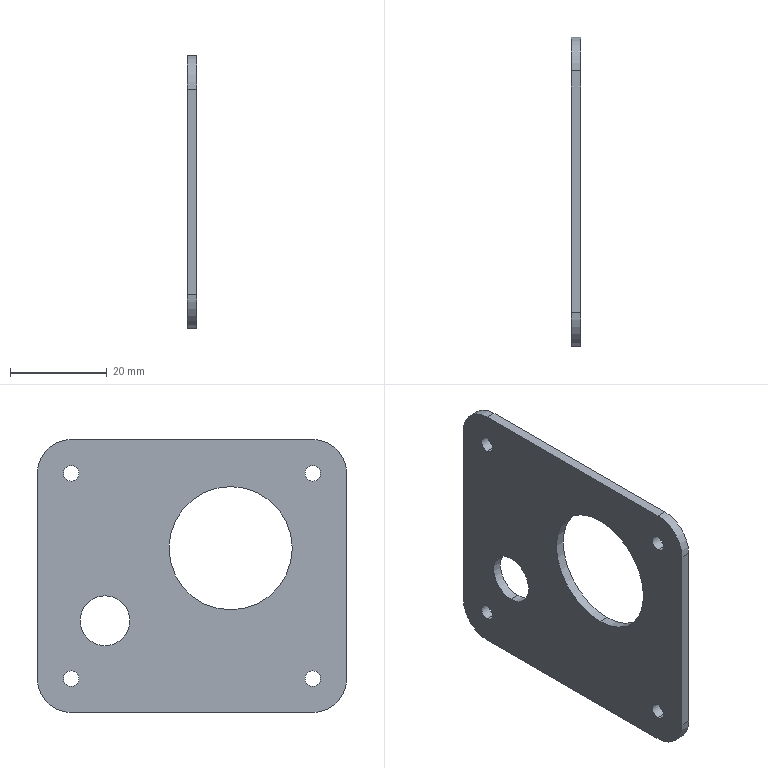Part | SolidWorks | features BaseBody 1 | 1 solid | 22 faces | box 2 x 64 x 56.5 mm | volume 5895 mm3 | cylinder 16 | plane 6 | commonest cylinder face diameters 3.2 x8 14 x4 10.3 x2 25.5 x2
STEP:
#1=CARTESIAN_POINT('',(-238.,130.5,52.4));
#2=VERTEX_POINT('',#1);
#3=CARTESIAN_POINT('',(-238.,130.5,55.6));
#4=VERTEX_POINT('',#3);
#5=CARTESIAN_POINT('',(-238.,130.5,54.));
#6=DIRECTION('',(-1.,0.,0.));
#7=DIRECTION('',(0.,0.,1.));
#8=AXIS2_PLACEMENT_3D('',#5,#6,#7);
#9=CIRCLE('',#8,1.6);
#10=EDGE_CURVE('',#2,#4,#9,.T.);
#11=ORIENTED_EDGE('',*,*,#10,.F.);
#12=CARTESIAN_POINT('',(-240.,130.5,52.4));
#13=VERTEX_POINT('',#12);
#14=CARTESIAN_POINT('',(-228.95,130.5,52.4));
#15=DIRECTION('',(-1.,0.,0.));
#16=VECTOR('',#15,1000.);
#17=LINE('',#14,#16);
#18=EDGE_CURVE('',#2,#13,#17,.T.);
#19=ORIENTED_EDGE('',*,*,#18,.T.);
#20=CARTESIAN_POINT('',(-240.,130.5,55.6));
#21=VERTEX_POINT('',#20);
#22=CARTESIAN_POINT('',(-240.,130.5,54.));
#23=DIRECTION('',(1.,0.,0.));
#24=DIRECTION('',(0.,0.,1.));
#25=AXIS2_PLACEMENT_3D('',#22,#23,#24);
#26=CIRCLE('',#25,1.6);
#27=EDGE_CURVE('',#21,#13,#26,.T.);
#28=ORIENTED_EDGE('',*,*,#27,.F.);
#29=CARTESIAN_POINT('',(-228.95,130.5,55.6));
#30=DIRECTION('',(-1.,0.,0.));
#31=VECTOR('',#30,1000.);
#32=LINE('',#29,#31);
#33=EDGE_CURVE('',#4,#21,#32,.T.);
#34=ORIENTED_EDGE('',*,*,#33,.F.);
#35=EDGE_LOOP('',(#11,#19,#28,#34));
#36=FACE_OUTER_BOUND('',#35,.T.);
#37=CARTESIAN_POINT('',(-228.95,130.5,54.));
#38=DIRECTION('',(-1.,0.,0.));
#39=DIRECTION('',(0.,0.,1.));
#40=AXIS2_PLACEMENT_3D('',#37,#38,#39);
#41=CYLINDRICAL_SURFACE('',#40,1.6);
#42=ADVANCED_FACE('',(#36),#41,.F.);
#43=CARTESIAN_POINT('',(-238.,80.5,9.9));
#44=VERTEX_POINT('',#43);
#45=CARTESIAN_POINT('',(-238.,80.5,13.1));
#46=VERTEX_POINT('',#45);
#47=CARTESIAN_POINT('',(-238.,80.5,11.5));
#48=DIRECTION('',(-1.,0.,0.));
#49=DIRECTION('',(0.,0.,1.));
#50=AXIS2_PLACEMENT_3D('',#47,#48,#49);
#51=CIRCLE('',#50,1.6);
#52=EDGE_CURVE('',#44,#46,#51,.T.);
#53=ORIENTED_EDGE('',*,*,#52,.F.);
#54=CARTESIAN_POINT('',(-240.,80.5,9.9));
#55=VERTEX_POINT('',#54);
#56=CARTESIAN_POINT('',(-228.95,80.5,9.9));
#57=DIRECTION('',(-1.,0.,0.));
#58=VECTOR('',#57,1000.);
#59=LINE('',#56,#58);
#60=EDGE_CURVE('',#44,#55,#59,.T.);
#61=ORIENTED_EDGE('',*,*,#60,.T.);
#62=CARTESIAN_POINT('',(-240.,80.5,13.1));
#63=VERTEX_POINT('',#62);
#64=CARTESIAN_POINT('',(-240.,80.5,11.5));
#65=DIRECTION('',(1.,0.,0.));
#66=DIRECTION('',(0.,0.,1.));
#67=AXIS2_PLACEMENT_3D('',#64,#65,#66);
#68=CIRCLE('',#67,1.6);
#69=EDGE_CURVE('',#63,#55,#68,.T.);
#70=ORIENTED_EDGE('',*,*,#69,.F.);
#71=CARTESIAN_POINT('',(-228.95,80.5,13.1));
#72=DIRECTION('',(-1.,0.,0.));
#73=VECTOR('',#72,1000.);
#74=LINE('',#71,#73);
#75=EDGE_CURVE('',#46,#63,#74,.T.);
#76=ORIENTED_EDGE('',*,*,#75,.F.);
#77=EDGE_LOOP('',(#53,#61,#70,#76));
#78=FACE_OUTER_BOUND('',#77,.T.);
#79=CARTESIAN_POINT('',(-228.95,80.5,11.5));
#80=DIRECTION('',(-1.,0.,0.));
#81=DIRECTION('',(0.,0.,1.));
#82=AXIS2_PLACEMENT_3D('',#79,#80,#81);
#83=CYLINDRICAL_SURFACE('',#82,1.6);
#84=ADVANCED_FACE('',(#78),#83,.F.);
#85=CARTESIAN_POINT('',(-238.,80.5,52.4));
#86=VERTEX_POINT('',#85);
#87=CARTESIAN_POINT('',(-238.,80.5,55.6));
#88=VERTEX_POINT('',#87);
#89=CARTESIAN_POINT('',(-238.,80.5,54.));
#90=DIRECTION('',(-1.,0.,0.));
#91=DIRECTION('',(0.,0.,1.));
#92=AXIS2_PLACEMENT_3D('',#89,#90,#91);
#93=CIRCLE('',#92,1.6);
#94=EDGE_CURVE('',#86,#88,#93,.T.);
#95=ORIENTED_EDGE('',*,*,#94,.F.);
#96=CARTESIAN_POINT('',(-240.,80.5,52.4));
#97=VERTEX_POINT('',#96);
#98=CARTESIAN_POINT('',(-228.95,80.5,52.4));
#99=DIRECTION('',(-1.,0.,0.));
#100=VECTOR('',#99,1000.);
#101=LINE('',#98,#100);
#102=EDGE_CURVE('',#86,#97,#101,.T.);
#103=ORIENTED_EDGE('',*,*,#102,.T.);
#104=CARTESIAN_POINT('',(-240.,80.5,55.6));
#105=VERTEX_POINT('',#104);
#106=CARTESIAN_POINT('',(-240.,80.5,54.));
#107=DIRECTION('',(1.,0.,0.));
#108=DIRECTION('',(0.,0.,1.));
#109=AXIS2_PLACEMENT_3D('',#106,#107,#108);
#110=CIRCLE('',#109,1.6);
#111=EDGE_CURVE('',#105,#97,#110,.T.);
#112=ORIENTED_EDGE('',*,*,#111,.F.);
#113=CARTESIAN_POINT('',(-228.95,80.5,55.6));
#114=DIRECTION('',(-1.,0.,0.));
#115=VECTOR('',#114,1000.);
#116=LINE('',#113,#115);
#117=EDGE_CURVE('',#88,#105,#116,.T.);
#118=ORIENTED_EDGE('',*,*,#117,.F.);
#119=EDGE_LOOP('',(#95,#103,#112,#118));
#120=FACE_OUTER_BOUND('',#119,.T.);
#121=CARTESIAN_POINT('',(-228.95,80.5,54.));
#122=DIRECTION('',(-1.,0.,0.));
#123=DIRECTION('',(0.,0.,1.));
#124=AXIS2_PLACEMENT_3D('',#121,#122,#123);
#125=CYLINDRICAL_SURFACE('',#124,1.6);
#126=ADVANCED_FACE('',(#120),#125,.F.);
#127=CARTESIAN_POINT('',(-238.,130.5,9.9));
#128=VERTEX_POINT('',#127);
#129=CARTESIAN_POINT('',(-238.,130.5,13.1));
#130=VERTEX_POINT('',#129);
#131=CARTESIAN_POINT('',(-238.,130.5,11.5));
#132=DIRECTION('',(-1.,0.,0.));
#133=DIRECTION('',(0.,0.,1.));
#134=AXIS2_PLACEMENT_3D('',#131,#132,#133);
#135=CIRCLE('',#134,1.6);
#136=EDGE_CURVE('',#128,#130,#135,.T.);
#137=ORIENTED_EDGE('',*,*,#136,.F.);
#138=CARTESIAN_POINT('',(-240.,130.5,9.9));
#139=VERTEX_POINT('',#138);
#140=CARTESIAN_POINT('',(-228.95,130.5,9.9));
#141=DIRECTION('',(-1.,0.,0.));
#142=VECTOR('',#141,1000.);
#143=LINE('',#140,#142);
#144=EDGE_CURVE('',#128,#139,#143,.T.);
#145=ORIENTED_EDGE('',*,*,#144,.T.);
#146=CARTESIAN_POINT('',(-240.,130.5,13.1));
#147=VERTEX_POINT('',#146);
#148=CARTESIAN_POINT('',(-240.,130.5,11.5));
#149=DIRECTION('',(1.,0.,0.));
#150=DIRECTION('',(0.,0.,1.));
#151=AXIS2_PLACEMENT_3D('',#148,#149,#150);
#152=CIRCLE('',#151,1.6);
#153=EDGE_CURVE('',#147,#139,#152,.T.);
#154=ORIENTED_EDGE('',*,*,#153,.F.);
#155=CARTESIAN_POINT('',(-228.95,130.5,13.1));
#156=DIRECTION('',(-1.,0.,0.));
#157=VECTOR('',#156,1000.);
#158=LINE('',#155,#157);
#159=EDGE_CURVE('',#130,#147,#158,.T.);
#160=ORIENTED_EDGE('',*,*,#159,.F.);
#161=EDGE_LOOP('',(#137,#145,#154,#160));
#162=FACE_OUTER_BOUND('',#161,.T.);
#163=CARTESIAN_POINT('',(-228.95,130.5,11.5));
#164=DIRECTION('',(-1.,0.,0.));
#165=DIRECTION('',(0.,0.,1.));
#166=AXIS2_PLACEMENT_3D('',#163,#164,#165);
#167=CYLINDRICAL_SURFACE('',#166,1.6);
#168=ADVANCED_FACE('',(#162),#167,.F.);
#169=CARTESIAN_POINT('',(-238.,123.5,18.35));
#170=VERTEX_POINT('',#169);
#171=CARTESIAN_POINT('',(-238.,123.5,28.65));
#172=VERTEX_POINT('',#171);
#173=CARTESIAN_POINT('',(-238.,123.5,23.5));
#174=DIRECTION('',(-1.,0.,0.));
#175=DIRECTION('',(0.,0.,1.));
#176=AXIS2_PLACEMENT_3D('',#173,#174,#175);
#177=CIRCLE('',#176,5.15);
#178=EDGE_CURVE('',#170,#172,#177,.T.);
#179=ORIENTED_EDGE('',*,*,#178,.F.);
#180=CARTESIAN_POINT('',(-240.,123.5,18.35));
#181=VERTEX_POINT('',#180);
#182=CARTESIAN_POINT('',(-140.,123.5,18.35));
#183=DIRECTION('',(-1.,0.,0.));
#184=VECTOR('',#183,1000.);
#185=LINE('',#182,#184);
#186=EDGE_CURVE('',#170,#181,#185,.T.);
#187=ORIENTED_EDGE('',*,*,#186,.T.);
#188=CARTESIAN_POINT('',(-240.,123.5,28.65));
#189=VERTEX_POINT('',#188);
#190=CARTESIAN_POINT('',(-240.,123.5,23.5));
#191=DIRECTION('',(1.,0.,0.));
#192=DIRECTION('',(0.,0.,1.));
#193=AXIS2_PLACEMENT_3D('',#190,#191,#192);
#194=CIRCLE('',#193,5.15);
#195=EDGE_CURVE('',#189,#181,#194,.T.);
#196=ORIENTED_EDGE('',*,*,#195,.F.);
#197=CARTESIAN_POINT('',(-140.,123.5,28.65));
#198=DIRECTION('',(-1.,0.,0.));
#199=VECTOR('',#198,1000.);
#200=LINE('',#197,#199);
#201=EDGE_CURVE('',#172,#189,#200,.T.);
#202=ORIENTED_EDGE('',*,*,#201,.F.);
#203=EDGE_LOOP('',(#179,#187,#196,#202));
#204=FACE_OUTER_BOUND('',#203,.T.);
#205=CARTESIAN_POINT('',(-140.,123.5,23.5));
#206=DIRECTION('',(-1.,0.,0.));
#207=DIRECTION('',(0.,0.,1.));
#208=AXIS2_PLACEMENT_3D('',#205,#206,#207);
#209=CYLINDRICAL_SURFACE('',#208,5.15);
#210=ADVANCED_FACE('',(#204),#209,.F.);
#211=CARTESIAN_POINT('',(-240.,97.5,51.25));
#212=VERTEX_POINT('',#211);
#213=CARTESIAN_POINT('',(-240.,97.5,25.75));
#214=VERTEX_POINT('',#213);
#215=CARTESIAN_POINT('',(-240.,97.5,38.5));
#216=DIRECTION('',(1.,0.,0.));
#217=DIRECTION('',(0.,0.,-1.));
#218=AXIS2_PLACEMENT_3D('',#215,#216,#217);
#219=CIRCLE('',#218,12.75);
#220=EDGE_CURVE('',#212,#214,#219,.T.);
#221=ORIENTED_EDGE('',*,*,#220,.F.);
#222=CARTESIAN_POINT('',(-238.,97.5,51.25));
#223=VERTEX_POINT('',#222);
#224=CARTESIAN_POINT('',(-279.,97.5,51.25));
#225=DIRECTION('',(1.,0.,0.));
#226=VECTOR('',#225,1000.);
#227=LINE('',#224,#226);
#228=EDGE_CURVE('',#212,#223,#227,.T.);
#229=ORIENTED_EDGE('',*,*,#228,.T.);
#230=CARTESIAN_POINT('',(-238.,97.5,25.75));
#231=VERTEX_POINT('',#230);
#232=CARTESIAN_POINT('',(-238.,97.5,38.5));
#233=DIRECTION('',(-1.,0.,0.));
#234=DIRECTION('',(0.,0.,-1.));
#235=AXIS2_PLACEMENT_3D('',#232,#233,#234);
#236=CIRCLE('',#235,12.75);
#237=EDGE_CURVE('',#231,#223,#236,.T.);
#238=ORIENTED_EDGE('',*,*,#237,.F.);
#239=CARTESIAN_POINT('',(-279.,97.5,25.75));
#240=DIRECTION('',(1.,0.,0.));
#241=VECTOR('',#240,1000.);
#242=LINE('',#239,#241);
#243=EDGE_CURVE('',#214,#231,#242,.T.);
#244=ORIENTED_EDGE('',*,*,#243,.F.);
#245=EDGE_LOOP('',(#221,#229,#238,#244));
#246=FACE_OUTER_BOUND('',#245,.T.);
#247=CARTESIAN_POINT('',(-279.,97.5,38.5));
#248=DIRECTION('',(1.,0.,0.));
#249=DIRECTION('',(0.,0.,-1.));
#250=AXIS2_PLACEMENT_3D('',#247,#248,#249);
#251=CYLINDRICAL_SURFACE('',#250,12.75);
#252=ADVANCED_FACE('',(#246),#251,.F.);
#253=CARTESIAN_POINT('',(-240.,97.5,38.5));
#254=DIRECTION('',(1.,0.,0.));
#255=DIRECTION('',(0.,0.,-1.));
#256=AXIS2_PLACEMENT_3D('',#253,#254,#255);
#257=CIRCLE('',#256,12.75);
#258=EDGE_CURVE('',#214,#212,#257,.T.);
#259=ORIENTED_EDGE('',*,*,#258,.T.);
#260=ORIENTED_EDGE('',*,*,#220,.T.);
#261=EDGE_LOOP('',(#259,#260));
#262=FACE_BOUND('',#261,.T.);
#263=ORIENTED_EDGE('',*,*,#195,.T.);
#264=CARTESIAN_POINT('',(-240.,123.5,23.5));
#265=DIRECTION('',(1.,0.,0.));
#266=DIRECTION('',(0.,0.,1.));
#267=AXIS2_PLACEMENT_3D('',#264,#265,#266);
#268=CIRCLE('',#267,5.15);
#269=EDGE_CURVE('',#181,#189,#268,.T.);
#270=ORIENTED_EDGE('',*,*,#269,.T.);
#271=EDGE_LOOP('',(#263,#270));
#272=FACE_BOUND('',#271,.T.);
#273=ORIENTED_EDGE('',*,*,#153,.T.);
#274=CARTESIAN_POINT('',(-240.,130.5,11.5));
#275=DIRECTION('',(1.,0.,0.));
#276=DIRECTION('',(0.,0.,1.));
#277=AXIS2_PLACEMENT_3D('',#274,#275,#276);
#278=CIRCLE('',#277,1.6);
#279=EDGE_CURVE('',#139,#147,#278,.T.);
#280=ORIENTED_EDGE('',*,*,#279,.T.);
#281=EDGE_LOOP('',(#273,#280));
#282=FACE_BOUND('',#281,.T.);
#283=ORIENTED_EDGE('',*,*,#111,.T.);
#284=CARTESIAN_POINT('',(-240.,80.5,54.));
#285=DIRECTION('',(1.,0.,0.));
#286=DIRECTION('',(0.,0.,1.));
#287=AXIS2_PLACEMENT_3D('',#284,#285,#286);
#288=CIRCLE('',#287,1.6);
#289=EDGE_CURVE('',#97,#105,#288,.T.);
#290=ORIENTED_EDGE('',*,*,#289,.T.);
#291=EDGE_LOOP('',(#283,#290));
#292=FACE_BOUND('',#291,.T.);
#293=ORIENTED_EDGE('',*,*,#69,.T.);
#294=CARTESIAN_POINT('',(-240.,80.5,11.5));
#295=DIRECTION('',(1.,0.,0.));
#296=DIRECTION('',(0.,0.,1.));
#297=AXIS2_PLACEMENT_3D('',#294,#295,#296);
#298=CIRCLE('',#297,1.6);
#299=EDGE_CURVE('',#55,#63,#298,.T.);
#300=ORIENTED_EDGE('',*,*,#299,.T.);
#301=EDGE_LOOP('',(#293,#300));
#302=FACE_BOUND('',#301,.T.);
#303=ORIENTED_EDGE('',*,*,#27,.T.);
#304=CARTESIAN_POINT('',(-240.,130.5,54.));
#305=DIRECTION('',(1.,0.,0.));
#306=DIRECTION('',(0.,0.,1.));
#307=AXIS2_PLACEMENT_3D('',#304,#305,#306);
#308=CIRCLE('',#307,1.6);
#309=EDGE_CURVE('',#13,#21,#308,.T.);
#310=ORIENTED_EDGE('',*,*,#309,.T.);
#311=EDGE_LOOP('',(#303,#310));
#312=FACE_BOUND('',#311,.T.);
#313=CARTESIAN_POINT('',(-240.,130.5,4.5));
#314=VERTEX_POINT('',#313);
#315=CARTESIAN_POINT('',(-240.,137.5,11.5));
#316=VERTEX_POINT('',#315);
#317=CARTESIAN_POINT('',(-240.,130.5,11.5));
#318=DIRECTION('',(1.,0.,0.));
#319=DIRECTION('',(0.,0.,1.));
#320=AXIS2_PLACEMENT_3D('',#317,#318,#319);
#321=CIRCLE('',#320,7.);
#322=EDGE_CURVE('',#314,#316,#321,.T.);
#323=ORIENTED_EDGE('',*,*,#322,.F.);
#324=CARTESIAN_POINT('',(-240.,80.5,4.5));
#325=VERTEX_POINT('',#324);
#326=CARTESIAN_POINT('',(-240.,94.5,4.5));
#327=DIRECTION('',(0.,-1.,0.));
#328=VECTOR('',#327,1000.);
#329=LINE('',#326,#328);
#330=EDGE_CURVE('',#314,#325,#329,.T.);
#331=ORIENTED_EDGE('',*,*,#330,.T.);
#332=CARTESIAN_POINT('',(-240.,73.5,11.5));
#333=VERTEX_POINT('',#332);
#334=CARTESIAN_POINT('',(-240.,80.5,11.5));
#335=DIRECTION('',(1.,0.,0.));
#336=DIRECTION('',(0.,0.,1.));
#337=AXIS2_PLACEMENT_3D('',#334,#335,#336);
#338=CIRCLE('',#337,7.);
#339=EDGE_CURVE('',#333,#325,#338,.T.);
#340=ORIENTED_EDGE('',*,*,#339,.F.);
#341=CARTESIAN_POINT('',(-240.,73.5,54.));
#342=VERTEX_POINT('',#341);
#343=CARTESIAN_POINT('',(-240.,73.5,48.5));
#344=DIRECTION('',(0.,0.,1.));
#345=VECTOR('',#344,1000.);
#346=LINE('',#343,#345);
#347=EDGE_CURVE('',#333,#342,#346,.T.);
#348=ORIENTED_EDGE('',*,*,#347,.T.);
#349=CARTESIAN_POINT('',(-240.,80.5,61.));
#350=VERTEX_POINT('',#349);
#351=CARTESIAN_POINT('',(-240.,80.5,54.));
#352=DIRECTION('',(1.,0.,0.));
#353=DIRECTION('',(0.,0.,1.));
#354=AXIS2_PLACEMENT_3D('',#351,#352,#353);
#355=CIRCLE('',#354,7.);
#356=EDGE_CURVE('',#350,#342,#355,.T.);
#357=ORIENTED_EDGE('',*,*,#356,.F.);
#358=CARTESIAN_POINT('',(-240.,130.5,61.));
#359=VERTEX_POINT('',#358);
#360=CARTESIAN_POINT('',(-240.,130.5,61.));
#361=DIRECTION('',(0.,1.,0.));
#362=VECTOR('',#361,1000.);
#363=LINE('',#360,#362);
#364=EDGE_CURVE('',#350,#359,#363,.T.);
#365=ORIENTED_EDGE('',*,*,#364,.T.);
#366=CARTESIAN_POINT('',(-240.,137.5,54.));
#367=VERTEX_POINT('',#366);
#368=CARTESIAN_POINT('',(-240.,130.5,54.));
#369=DIRECTION('',(1.,0.,0.));
#370=DIRECTION('',(0.,0.,1.));
#371=AXIS2_PLACEMENT_3D('',#368,#369,#370);
#372=CIRCLE('',#371,7.);
#373=EDGE_CURVE('',#367,#359,#372,.T.);
#374=ORIENTED_EDGE('',*,*,#373,.F.);
#375=CARTESIAN_POINT('',(-240.,137.5,13.5));
#376=DIRECTION('',(0.,0.,-1.));
#377=VECTOR('',#376,1000.);
#378=LINE('',#375,#377);
#379=EDGE_CURVE('',#367,#316,#378,.T.);
#380=ORIENTED_EDGE('',*,*,#379,.T.);
#381=EDGE_LOOP('',(#323,#331,#340,#348,#357,#365,#374,#380));
#382=FACE_OUTER_BOUND('',#381,.T.);
#383=CARTESIAN_POINT('',(-240.,130.5,48.5));
#384=DIRECTION('',(1.,0.,0.));
#385=DIRECTION('',(0.,1.,0.));
#386=AXIS2_PLACEMENT_3D('',#383,#384,#385);
#387=PLANE('',#386);
#388=ADVANCED_FACE('',(#262,#272,#282,#292,#302,#312,#382),#387,.F.);
#389=ORIENTED_EDGE('',*,*,#322,.T.);
#390=CARTESIAN_POINT('',(-238.,137.5,11.5));
#391=VERTEX_POINT('',#390);
#392=CARTESIAN_POINT('',(-238.,137.5,11.5));
#393=DIRECTION('',(1.,0.,0.));
#394=VECTOR('',#393,1000.);
#395=LINE('',#392,#394);
#396=EDGE_CURVE('',#316,#391,#395,.T.);
#397=ORIENTED_EDGE('',*,*,#396,.T.);
#398=CARTESIAN_POINT('',(-238.,130.5,4.5));
#399=VERTEX_POINT('',#398);
#400=CARTESIAN_POINT('',(-238.,130.5,11.5));
#401=DIRECTION('',(1.,0.,0.));
#402=DIRECTION('',(0.,0.,1.));
#403=AXIS2_PLACEMENT_3D('',#400,#401,#402);
#404=CIRCLE('',#403,7.);
#405=EDGE_CURVE('',#399,#391,#404,.T.);
#406=ORIENTED_EDGE('',*,*,#405,.F.);
#407=CARTESIAN_POINT('',(-238.,130.5,4.5));
#408=DIRECTION('',(-1.,0.,0.));
#409=VECTOR('',#408,1000.);
#410=LINE('',#407,#409);
#411=EDGE_CURVE('',#399,#314,#410,.T.);
#412=ORIENTED_EDGE('',*,*,#411,.T.);
#413=EDGE_LOOP('',(#389,#397,#406,#412));
#414=FACE_OUTER_BOUND('',#413,.T.);
#415=CARTESIAN_POINT('',(-238.,130.5,11.5));
#416=DIRECTION('',(-1.,0.,0.));
#417=DIRECTION('',(0.,0.,1.));
#418=AXIS2_PLACEMENT_3D('',#415,#416,#417);
#419=CYLINDRICAL_SURFACE('',#418,7.);
#420=ADVANCED_FACE('',(#414),#419,.T.);
#421=CARTESIAN_POINT('',(-238.,137.5,54.));
#422=VERTEX_POINT('',#421);
#423=CARTESIAN_POINT('',(-238.,137.5,48.5));
#424=DIRECTION('',(0.,0.,1.));
#425=VECTOR('',#424,1000.);
#426=LINE('',#423,#425);
#427=EDGE_CURVE('',#391,#422,#426,.T.);
#428=ORIENTED_EDGE('',*,*,#427,.F.);
#429=ORIENTED_EDGE('',*,*,#396,.F.);
#430=ORIENTED_EDGE('',*,*,#379,.F.);
#431=CARTESIAN_POINT('',(-238.,137.5,54.));
#432=DIRECTION('',(-1.,0.,0.));
#433=VECTOR('',#432,1000.);
#434=LINE('',#431,#433);
#435=EDGE_CURVE('',#422,#367,#434,.T.);
#436=ORIENTED_EDGE('',*,*,#435,.F.);
#437=EDGE_LOOP('',(#428,#429,#430,#436));
#438=FACE_OUTER_BOUND('',#437,.T.);
#439=CARTESIAN_POINT('',(-238.,137.5,13.5));
#440=DIRECTION('',(0.,-1.,0.));
#441=DIRECTION('',(0.,0.,-1.));
#442=AXIS2_PLACEMENT_3D('',#439,#440,#441);
#443=PLANE('',#442);
#444=ADVANCED_FACE('',(#438),#443,.F.);
#445=ORIENTED_EDGE('',*,*,#373,.T.);
#446=CARTESIAN_POINT('',(-238.,130.5,61.));
#447=VERTEX_POINT('',#446);
#448=CARTESIAN_POINT('',(-238.,130.5,61.));
#449=DIRECTION('',(1.,0.,0.));
#450=VECTOR('',#449,1000.);
#451=LINE('',#448,#450);
#452=EDGE_CURVE('',#359,#447,#451,.T.);
#453=ORIENTED_EDGE('',*,*,#452,.T.);
#454=CARTESIAN_POINT('',(-238.,130.5,54.));
#455=DIRECTION('',(1.,0.,0.));
#456=DIRECTION('',(0.,0.,1.));
#457=AXIS2_PLACEMENT_3D('',#454,#455,#456);
#458=CIRCLE('',#457,7.);
#459=EDGE_CURVE('',#422,#447,#458,.T.);
#460=ORIENTED_EDGE('',*,*,#459,.F.);
#461=ORIENTED_EDGE('',*,*,#435,.T.);
#462=EDGE_LOOP('',(#445,#453,#460,#461));
#463=FACE_OUTER_BOUND('',#462,.T.);
#464=CARTESIAN_POINT('',(-238.,130.5,54.));
#465=DIRECTION('',(-1.,0.,0.));
#466=DIRECTION('',(0.,0.,1.));
#467=AXIS2_PLACEMENT_3D('',#464,#465,#466);
#468=CYLINDRICAL_SURFACE('',#467,7.);
#469=ADVANCED_FACE('',(#463),#468,.T.);
#470=CARTESIAN_POINT('',(-238.,80.5,61.));
#471=VERTEX_POINT('',#470);
#472=CARTESIAN_POINT('',(-238.,130.5,61.));
#473=DIRECTION('',(0.,-1.,0.));
#474=VECTOR('',#473,1000.);
#475=LINE('',#472,#474);
#476=EDGE_CURVE('',#447,#471,#475,.T.);
#477=ORIENTED_EDGE('',*,*,#476,.F.);
#478=ORIENTED_EDGE('',*,*,#452,.F.);
#479=ORIENTED_EDGE('',*,*,#364,.F.);
#480=CARTESIAN_POINT('',(-238.,80.5,61.));
#481=DIRECTION('',(-1.,0.,0.));
#482=VECTOR('',#481,1000.);
#483=LINE('',#480,#482);
#484=EDGE_CURVE('',#471,#350,#483,.T.);
#485=ORIENTED_EDGE('',*,*,#484,.F.);
#486=EDGE_LOOP('',(#477,#478,#479,#485));
#487=FACE_OUTER_BOUND('',#486,.T.);
#488=CARTESIAN_POINT('',(-238.,130.5,61.));
#489=DIRECTION('',(0.,0.,-1.));
#490=DIRECTION('',(0.,-1.,0.));
#491=AXIS2_PLACEMENT_3D('',#488,#489,#490);
#492=PLANE('',#491);
#493=ADVANCED_FACE('',(#487),#492,.F.);
#494=ORIENTED_EDGE('',*,*,#356,.T.);
#495=CARTESIAN_POINT('',(-238.,73.5,54.));
#496=VERTEX_POINT('',#495);
#497=CARTESIAN_POINT('',(-238.,73.5,54.));
#498=DIRECTION('',(1.,0.,0.));
#499=VECTOR('',#498,1000.);
#500=LINE('',#497,#499);
#501=EDGE_CURVE('',#342,#496,#500,.T.);
#502=ORIENTED_EDGE('',*,*,#501,.T.);
#503=CARTESIAN_POINT('',(-238.,80.5,54.));
#504=DIRECTION('',(1.,0.,0.));
#505=DIRECTION('',(0.,0.,1.));
#506=AXIS2_PLACEMENT_3D('',#503,#504,#505);
#507=CIRCLE('',#506,7.);
#508=EDGE_CURVE('',#471,#496,#507,.T.);
#509=ORIENTED_EDGE('',*,*,#508,.F.);
#510=ORIENTED_EDGE('',*,*,#484,.T.);
#511=EDGE_LOOP('',(#494,#502,#509,#510));
#512=FACE_OUTER_BOUND('',#511,.T.);
#513=CARTESIAN_POINT('',(-238.,80.5,54.));
#514=DIRECTION('',(-1.,0.,0.));
#515=DIRECTION('',(0.,0.,1.));
#516=AXIS2_PLACEMENT_3D('',#513,#514,#515);
#517=CYLINDRICAL_SURFACE('',#516,7.);
#518=ADVANCED_FACE('',(#512),#517,.T.);
#519=CARTESIAN_POINT('',(-238.,73.5,11.5));
#520=VERTEX_POINT('',#519);
#521=CARTESIAN_POINT('',(-238.,73.5,48.5));
#522=DIRECTION('',(0.,0.,-1.));
#523=VECTOR('',#522,1000.);
#524=LINE('',#521,#523);
#525=EDGE_CURVE('',#496,#520,#524,.T.);
#526=ORIENTED_EDGE('',*,*,#525,.F.);
#527=ORIENTED_EDGE('',*,*,#501,.F.);
#528=ORIENTED_EDGE('',*,*,#347,.F.);
#529=CARTESIAN_POINT('',(-238.,73.5,11.5));
#530=DIRECTION('',(-1.,0.,0.));
#531=VECTOR('',#530,1000.);
#532=LINE('',#529,#531);
#533=EDGE_CURVE('',#520,#333,#532,.T.);
#534=ORIENTED_EDGE('',*,*,#533,.F.);
#535=EDGE_LOOP('',(#526,#527,#528,#534));
#536=FACE_OUTER_BOUND('',#535,.T.);
#537=CARTESIAN_POINT('',(-238.,73.5,48.5));
#538=DIRECTION('',(0.,1.,0.));
#539=DIRECTION('',(1.,0.,0.));
#540=AXIS2_PLACEMENT_3D('',#537,#538,#539);
#541=PLANE('',#540);
#542=ADVANCED_FACE('',(#536),#541,.F.);
#543=ORIENTED_EDGE('',*,*,#339,.T.);
#544=CARTESIAN_POINT('',(-238.,80.5,4.5));
#545=VERTEX_POINT('',#544);
#546=CARTESIAN_POINT('',(-238.,80.5,4.5));
#547=DIRECTION('',(1.,0.,0.));
#548=VECTOR('',#547,1000.);
#549=LINE('',#546,#548);
#550=EDGE_CURVE('',#325,#545,#549,.T.);
#551=ORIENTED_EDGE('',*,*,#550,.T.);
#552=CARTESIAN_POINT('',(-238.,80.5,11.5));
#553=DIRECTION('',(1.,0.,0.));
#554=DIRECTION('',(0.,0.,1.));
#555=AXIS2_PLACEMENT_3D('',#552,#553,#554);
#556=CIRCLE('',#555,7.);
#557=EDGE_CURVE('',#520,#545,#556,.T.);
#558=ORIENTED_EDGE('',*,*,#557,.F.);
#559=ORIENTED_EDGE('',*,*,#533,.T.);
#560=EDGE_LOOP('',(#543,#551,#558,#559));
#561=FACE_OUTER_BOUND('',#560,.T.);
#562=CARTESIAN_POINT('',(-238.,80.5,11.5));
#563=DIRECTION('',(-1.,0.,0.));
#564=DIRECTION('',(0.,0.,1.));
#565=AXIS2_PLACEMENT_3D('',#562,#563,#564);
#566=CYLINDRICAL_SURFACE('',#565,7.);
#567=ADVANCED_FACE('',(#561),#566,.T.);
#568=CARTESIAN_POINT('',(-238.,130.5,4.5));
#569=DIRECTION('',(0.,1.,0.));
#570=VECTOR('',#569,1000.);
#571=LINE('',#568,#570);
#572=EDGE_CURVE('',#545,#399,#571,.T.);
#573=ORIENTED_EDGE('',*,*,#572,.F.);
#574=ORIENTED_EDGE('',*,*,#550,.F.);
#575=ORIENTED_EDGE('',*,*,#330,.F.);
#576=ORIENTED_EDGE('',*,*,#411,.F.);
#577=EDGE_LOOP('',(#573,#574,#575,#576));
#578=FACE_OUTER_BOUND('',#577,.T.);
#579=CARTESIAN_POINT('',(-238.,94.5,4.5));
#580=DIRECTION('',(0.,0.,1.));
#581=DIRECTION('',(1.,0.,0.));
#582=AXIS2_PLACEMENT_3D('',#579,#580,#581);
#583=PLANE('',#582);
#584=ADVANCED_FACE('',(#578),#583,.F.);
#585=ORIENTED_EDGE('',*,*,#237,.T.);
#586=CARTESIAN_POINT('',(-238.,97.5,38.5));
#587=DIRECTION('',(-1.,0.,0.));
#588=DIRECTION('',(0.,0.,-1.));
#589=AXIS2_PLACEMENT_3D('',#586,#587,#588);
#590=CIRCLE('',#589,12.75);
#591=EDGE_CURVE('',#223,#231,#590,.T.);
#592=ORIENTED_EDGE('',*,*,#591,.T.);
#593=EDGE_LOOP('',(#585,#592));
#594=FACE_BOUND('',#593,.T.);
#595=CARTESIAN_POINT('',(-238.,123.5,23.5));
#596=DIRECTION('',(-1.,0.,0.));
#597=DIRECTION('',(0.,0.,1.));
#598=AXIS2_PLACEMENT_3D('',#595,#596,#597);
#599=CIRCLE('',#598,5.15);
#600=EDGE_CURVE('',#172,#170,#599,.T.);
#601=ORIENTED_EDGE('',*,*,#600,.T.);
#602=ORIENTED_EDGE('',*,*,#178,.T.);
#603=EDGE_LOOP('',(#601,#602));
#604=FACE_BOUND('',#603,.T.);
#605=CARTESIAN_POINT('',(-238.,130.5,11.5));
#606=DIRECTION('',(-1.,0.,0.));
#607=DIRECTION('',(0.,0.,1.));
#608=AXIS2_PLACEMENT_3D('',#605,#606,#607);
#609=CIRCLE('',#608,1.6);
#610=EDGE_CURVE('',#130,#128,#609,.T.);
#611=ORIENTED_EDGE('',*,*,#610,.T.);
#612=ORIENTED_EDGE('',*,*,#136,.T.);
#613=EDGE_LOOP('',(#611,#612));
#614=FACE_BOUND('',#613,.T.);
#615=CARTESIAN_POINT('',(-238.,80.5,54.));
#616=DIRECTION('',(-1.,0.,0.));
#617=DIRECTION('',(0.,0.,1.));
#618=AXIS2_PLACEMENT_3D('',#615,#616,#617);
#619=CIRCLE('',#618,1.6);
#620=EDGE_CURVE('',#88,#86,#619,.T.);
#621=ORIENTED_EDGE('',*,*,#620,.T.);
#622=ORIENTED_EDGE('',*,*,#94,.T.);
#623=EDGE_LOOP('',(#621,#622));
#624=FACE_BOUND('',#623,.T.);
#625=CARTESIAN_POINT('',(-238.,80.5,11.5));
#626=DIRECTION('',(-1.,0.,0.));
#627=DIRECTION('',(0.,0.,1.));
#628=AXIS2_PLACEMENT_3D('',#625,#626,#627);
#629=CIRCLE('',#628,1.6);
#630=EDGE_CURVE('',#46,#44,#629,.T.);
#631=ORIENTED_EDGE('',*,*,#630,.T.);
#632=ORIENTED_EDGE('',*,*,#52,.T.);
#633=EDGE_LOOP('',(#631,#632));
#634=FACE_BOUND('',#633,.T.);
#635=CARTESIAN_POINT('',(-238.,130.5,54.));
#636=DIRECTION('',(-1.,0.,0.));
#637=DIRECTION('',(0.,0.,1.));
#638=AXIS2_PLACEMENT_3D('',#635,#636,#637);
#639=CIRCLE('',#638,1.6);
#640=EDGE_CURVE('',#4,#2,#639,.T.);
#641=ORIENTED_EDGE('',*,*,#640,.T.);
#642=ORIENTED_EDGE('',*,*,#10,.T.);
#643=EDGE_LOOP('',(#641,#642));
#644=FACE_BOUND('',#643,.T.);
#645=ORIENTED_EDGE('',*,*,#557,.T.);
#646=ORIENTED_EDGE('',*,*,#572,.T.);
#647=ORIENTED_EDGE('',*,*,#405,.T.);
#648=ORIENTED_EDGE('',*,*,#427,.T.);
#649=ORIENTED_EDGE('',*,*,#459,.T.);
#650=ORIENTED_EDGE('',*,*,#476,.T.);
#651=ORIENTED_EDGE('',*,*,#508,.T.);
#652=ORIENTED_EDGE('',*,*,#525,.T.);
#653=EDGE_LOOP('',(#645,#646,#647,#648,#649,#650,#651,#652));
#654=FACE_OUTER_BOUND('',#653,.T.);
#655=CARTESIAN_POINT('',(-238.,130.5,48.5));
#656=DIRECTION('',(1.,0.,0.));
#657=DIRECTION('',(0.,1.,0.));
#658=AXIS2_PLACEMENT_3D('',#655,#656,#657);
#659=PLANE('',#658);
#660=ADVANCED_FACE('',(#594,#604,#614,#624,#634,#644,#654),#659,.T.);
#661=ORIENTED_EDGE('',*,*,#228,.F.);
#662=ORIENTED_EDGE('',*,*,#258,.F.);
#663=ORIENTED_EDGE('',*,*,#243,.T.);
#664=ORIENTED_EDGE('',*,*,#591,.F.);
#665=EDGE_LOOP('',(#661,#662,#663,#664));
#666=FACE_OUTER_BOUND('',#665,.T.);
#667=CARTESIAN_POINT('',(-279.,97.5,38.5));
#668=DIRECTION('',(1.,0.,0.));
#669=DIRECTION('',(0.,0.,-1.));
#670=AXIS2_PLACEMENT_3D('',#667,#668,#669);
#671=CYLINDRICAL_SURFACE('',#670,12.75);
#672=ADVANCED_FACE('',(#666),#671,.F.);
#673=ORIENTED_EDGE('',*,*,#186,.F.);
#674=ORIENTED_EDGE('',*,*,#600,.F.);
#675=ORIENTED_EDGE('',*,*,#201,.T.);
#676=ORIENTED_EDGE('',*,*,#269,.F.);
#677=EDGE_LOOP('',(#673,#674,#675,#676));
#678=FACE_OUTER_BOUND('',#677,.T.);
#679=CARTESIAN_POINT('',(-140.,123.5,23.5));
#680=DIRECTION('',(-1.,0.,0.));
#681=DIRECTION('',(0.,0.,1.));
#682=AXIS2_PLACEMENT_3D('',#679,#680,#681);
#683=CYLINDRICAL_SURFACE('',#682,5.15);
#684=ADVANCED_FACE('',(#678),#683,.F.);
#685=ORIENTED_EDGE('',*,*,#144,.F.);
#686=ORIENTED_EDGE('',*,*,#610,.F.);
#687=ORIENTED_EDGE('',*,*,#159,.T.);
#688=ORIENTED_EDGE('',*,*,#279,.F.);
#689=EDGE_LOOP('',(#685,#686,#687,#688));
#690=FACE_OUTER_BOUND('',#689,.T.);
#691=CARTESIAN_POINT('',(-228.95,130.5,11.5));
#692=DIRECTION('',(-1.,0.,0.));
#693=DIRECTION('',(0.,0.,1.));
#694=AXIS2_PLACEMENT_3D('',#691,#692,#693);
#695=CYLINDRICAL_SURFACE('',#694,1.6);
#696=ADVANCED_FACE('',(#690),#695,.F.);
#697=ORIENTED_EDGE('',*,*,#102,.F.);
#698=ORIENTED_EDGE('',*,*,#620,.F.);
#699=ORIENTED_EDGE('',*,*,#117,.T.);
#700=ORIENTED_EDGE('',*,*,#289,.F.);
#701=EDGE_LOOP('',(#697,#698,#699,#700));
#702=FACE_OUTER_BOUND('',#701,.T.);
#703=CARTESIAN_POINT('',(-228.95,80.5,54.));
#704=DIRECTION('',(-1.,0.,0.));
#705=DIRECTION('',(0.,0.,1.));
#706=AXIS2_PLACEMENT_3D('',#703,#704,#705);
#707=CYLINDRICAL_SURFACE('',#706,1.6);
#708=ADVANCED_FACE('',(#702),#707,.F.);
#709=ORIENTED_EDGE('',*,*,#60,.F.);
#710=ORIENTED_EDGE('',*,*,#630,.F.);
#711=ORIENTED_EDGE('',*,*,#75,.T.);
#712=ORIENTED_EDGE('',*,*,#299,.F.);
#713=EDGE_LOOP('',(#709,#710,#711,#712));
#714=FACE_OUTER_BOUND('',#713,.T.);
#715=CARTESIAN_POINT('',(-228.95,80.5,11.5));
#716=DIRECTION('',(-1.,0.,0.));
#717=DIRECTION('',(0.,0.,1.));
#718=AXIS2_PLACEMENT_3D('',#715,#716,#717);
#719=CYLINDRICAL_SURFACE('',#718,1.6);
#720=ADVANCED_FACE('',(#714),#719,.F.);
#721=ORIENTED_EDGE('',*,*,#18,.F.);
#722=ORIENTED_EDGE('',*,*,#640,.F.);
#723=ORIENTED_EDGE('',*,*,#33,.T.);
#724=ORIENTED_EDGE('',*,*,#309,.F.);
#725=EDGE_LOOP('',(#721,#722,#723,#724));
#726=FACE_OUTER_BOUND('',#725,.T.);
#727=CARTESIAN_POINT('',(-228.95,130.5,54.));
#728=DIRECTION('',(-1.,0.,0.));
#729=DIRECTION('',(0.,0.,1.));
#730=AXIS2_PLACEMENT_3D('',#727,#728,#729);
#731=CYLINDRICAL_SURFACE('',#730,1.6);
#732=ADVANCED_FACE('',(#726),#731,.F.);
#733=CLOSED_SHELL('',(#42,#84,#126,#168,#210,#252,#388,#420,#444,#469,#493,#518,#542,#567,#584,#660,#672,#684,#696,#708,#720,#732));
#734=MANIFOLD_SOLID_BREP('',#733);
#735=CARTESIAN_POINT('',(0.,0.,0.));
#736=DIRECTION('',(0.,0.,1.));
#737=DIRECTION('',(1.,0.,0.));
#738=AXIS2_PLACEMENT_3D('',#735,#736,#737);
#739=(LENGTH_UNIT()NAMED_UNIT(*)SI_UNIT(.MILLI.,.METRE.));
#740=UNCERTAINTY_MEASURE_WITH_UNIT(LENGTH_MEASURE(0.00001),#739,'','');
#741=(NAMED_UNIT(*)PLANE_ANGLE_UNIT()SI_UNIT($,.RADIAN.));
#742=(NAMED_UNIT(*)SI_UNIT($,.STERADIAN.)SOLID_ANGLE_UNIT());
#743=(GEOMETRIC_REPRESENTATION_CONTEXT(3)GLOBAL_UNCERTAINTY_ASSIGNED_CONTEXT((#740))GLOBAL_UNIT_ASSIGNED_CONTEXT((#739,#741,#742))REPRESENTATION_CONTEXT('',''));
#744=ADVANCED_BREP_SHAPE_REPRESENTATION('',(#734,#738),#743);